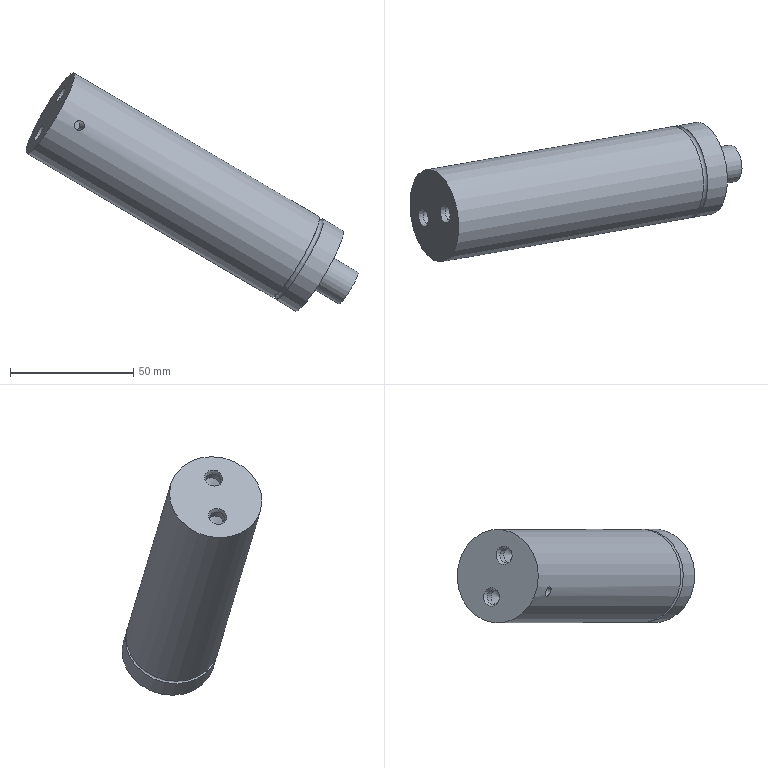Part | NX | features solid 2 | 1 solid | 15 faces | box 134.944 x 56.817 x 96.909 mm | volume 146987 mm3 | cylinder 7 | cone 4 | plane 3 | torus 1 | commonest cylinder face diameters 6 x2 38 x2 4 x1 15 x1 18 x1
STEP:
#1=CARTESIAN_POINT('',(878.455,397.185,19.862));
#2=VERTEX_POINT('',#1);
#3=CARTESIAN_POINT('',(877.303,397.035,18.721));
#4=CARTESIAN_POINT('',(878.645,397.191,19.754));
#5=CARTESIAN_POINT('',(878.849,397.307,21.436));
#6=CARTESIAN_POINT('',(877.82,397.207,22.781));
#7=CARTESIAN_POINT('',(876.177,396.836,23.005));
#8=CARTESIAN_POINT('',(874.865,396.525,21.972));
#9=CARTESIAN_POINT('',(874.632,396.564,20.293));
#10=CARTESIAN_POINT('',(875.633,396.821,18.945));
#11=CARTESIAN_POINT('',(877.303,397.035,18.721));
#12=CARTESIAN_POINT('',(878.645,397.191,19.754));
#13=CARTESIAN_POINT('',(878.849,397.307,21.436));
#14=B_SPLINE_CURVE_WITH_KNOTS('',3,(#3,#4,#5,#6,#7,#8,#9,#10,#11,#12,#13),.UNSPECIFIED.,.T.,.F.,(1,1,1,1,1,1,1,1,1,1,1,1,1,1,1),(-0.004692,-0.003128,-0.001564,0.,0.001564,0.003128,0.004692,0.006257,0.007821,0.009385,0.01095,0.01251,0.01408,0.01564,0.01721),.UNSPECIFIED.);
#15=EDGE_CURVE('',#2,#2,#14,.T.);
#16=ORIENTED_EDGE('',*,*,#15,.F.);
#17=EDGE_LOOP('',(#16));
#18=FACE_BOUND('',#17,.T.);
#19=CARTESIAN_POINT('',(855.566,412.442,9.408));
#20=VERTEX_POINT('',#19);
#21=CARTESIAN_POINT('',(864.922,414.091,25.863));
#22=DIRECTION('',(0.8529,0.1504,-0.5));
#23=DIRECTION('',(-0.4924,-0.08682,-0.866));
#24=AXIS2_PLACEMENT_3D('',#21,#22,#23);
#25=CIRCLE('',#24,19.);
#26=EDGE_CURVE('',#20,#20,#25,.T.);
#27=ORIENTED_EDGE('',*,*,#26,.T.);
#28=EDGE_LOOP('',(#27));
#29=FACE_BOUND('',#28,.T.);
#30=CARTESIAN_POINT('',(955.011,429.976,-48.892));
#31=VERTEX_POINT('',#30);
#32=CARTESIAN_POINT('',(964.366,431.626,-32.437));
#33=DIRECTION('',(0.8529,0.1504,-0.5));
#34=DIRECTION('',(-0.4924,-0.08682,-0.866));
#35=AXIS2_PLACEMENT_3D('',#32,#33,#34);
#36=CIRCLE('',#35,19.);
#37=EDGE_CURVE('',#31,#31,#36,.T.);
#38=ORIENTED_EDGE('',*,*,#37,.F.);
#39=EDGE_LOOP('',(#38));
#40=FACE_BOUND('',#39,.T.);
#41=CARTESIAN_POINT('',(972.81,433.115,-37.387));
#42=DIRECTION('',(-0.8529,-0.1504,0.5));
#43=DIRECTION('',(0.4924,0.08682,0.866));
#44=AXIS2_PLACEMENT_3D('',#41,#42,#43);
#45=CYLINDRICAL_SURFACE('',#44,19.);
#46=ADVANCED_FACE('',(#18,#29,#40),#45,.T.);
#47=CARTESIAN_POINT('',(867.507,414.547,30.41));
#48=VERTEX_POINT('',#47);
#49=CARTESIAN_POINT('',(869.353,414.873,33.657));
#50=DIRECTION('',(-0.8529,-0.1504,0.5));
#51=DIRECTION('',(-0.4924,-0.08682,-0.866));
#52=AXIS2_PLACEMENT_3D('',#49,#50,#51);
#53=CIRCLE('',#52,3.75);
#54=EDGE_CURVE('',#48,#48,#53,.T.);
#55=ORIENTED_EDGE('',*,*,#54,.F.);
#56=EDGE_LOOP('',(#55));
#57=FACE_BOUND('',#56,.T.);
#58=CARTESIAN_POINT('',(858.644,412.984,14.821));
#59=VERTEX_POINT('',#58);
#60=CARTESIAN_POINT('',(860.49,413.31,18.069));
#61=DIRECTION('',(-0.8529,-0.1504,0.5));
#62=DIRECTION('',(-0.4924,-0.08682,-0.866));
#63=AXIS2_PLACEMENT_3D('',#60,#61,#62);
#64=CIRCLE('',#63,3.75);
#65=EDGE_CURVE('',#59,#59,#64,.T.);
#66=ORIENTED_EDGE('',*,*,#65,.F.);
#67=EDGE_LOOP('',(#66));
#68=FACE_BOUND('',#67,.T.);
#69=ORIENTED_EDGE('',*,*,#26,.F.);
#70=EDGE_LOOP('',(#69));
#71=FACE_BOUND('',#70,.T.);
#72=CARTESIAN_POINT('',(864.922,414.091,25.863));
#73=DIRECTION('',(-0.8529,-0.1504,0.5));
#74=DIRECTION('',(0.4924,0.08682,0.866));
#75=AXIS2_PLACEMENT_3D('',#72,#73,#74);
#76=PLANE('',#75);
#77=ADVANCED_FACE('',(#57,#68,#71),#76,.T.);
#78=ORIENTED_EDGE('',*,*,#15,.T.);
#79=EDGE_LOOP('',(#78));
#80=FACE_BOUND('',#79,.T.);
#81=CARTESIAN_POINT('',(876.826,407.055,20.081));
#82=VERTEX_POINT('',#81);
#83=CARTESIAN_POINT('',(877.011,407.239,21.692));
#84=CARTESIAN_POINT('',(877.032,407.036,19.997));
#85=CARTESIAN_POINT('',(875.815,406.945,18.807));
#86=CARTESIAN_POINT('',(874.114,406.854,18.822));
#87=CARTESIAN_POINT('',(872.962,406.524,20.036));
#88=CARTESIAN_POINT('',(873.013,406.328,21.728));
#89=CARTESIAN_POINT('',(874.184,406.657,22.918));
#90=CARTESIAN_POINT('',(875.817,407.155,22.904));
#91=CARTESIAN_POINT('',(877.011,407.239,21.692));
#92=CARTESIAN_POINT('',(877.032,407.036,19.997));
#93=CARTESIAN_POINT('',(875.815,406.945,18.807));
#94=B_SPLINE_CURVE_WITH_KNOTS('',3,(#83,#84,#85,#86,#87,#88,#89,#90,#91,#92,#93),.UNSPECIFIED.,.T.,.F.,(1,1,1,1,1,1,1,1,1,1,1,1,1,1,1),(-0.004704,-0.003136,-0.001568,0.,0.001568,0.003136,0.004704,0.006272,0.00784,0.009408,0.01098,0.01254,0.01411,0.01568,0.01725),.UNSPECIFIED.);
#95=EDGE_CURVE('',#82,#82,#94,.T.);
#96=ORIENTED_EDGE('',*,*,#95,.T.);
#97=EDGE_LOOP('',(#96));
#98=FACE_BOUND('',#97,.T.);
#99=CARTESIAN_POINT('',(879.007,384.081,20.863));
#100=DIRECTION('',(-0.1736,0.9848,0.));
#101=DIRECTION('',(-0.4924,-0.08682,-0.866));
#102=AXIS2_PLACEMENT_3D('',#99,#100,#101);
#103=CYLINDRICAL_SURFACE('',#102,2.);
#104=ADVANCED_FACE('',(#80,#98),#103,.F.);
#105=CARTESIAN_POINT('',(863.277,413.801,12.971));
#106=VERTEX_POINT('',#105);
#107=CARTESIAN_POINT('',(864.755,414.062,15.569));
#108=DIRECTION('',(-0.8529,-0.1504,0.5));
#109=DIRECTION('',(-0.4924,-0.08682,-0.866));
#110=AXIS2_PLACEMENT_3D('',#107,#108,#109);
#111=CIRCLE('',#110,3.);
#112=EDGE_CURVE('',#106,#106,#111,.T.);
#113=ORIENTED_EDGE('',*,*,#112,.T.);
#114=EDGE_LOOP('',(#113));
#115=FACE_BOUND('',#114,.T.);
#116=CARTESIAN_POINT('',(866.292,414.333,14.667));
#117=VERTEX_POINT('',#116);
#118=VERTEX_LOOP('',#117);
#119=FACE_BOUND('',#118,.T.);
#120=CARTESIAN_POINT('',(864.755,414.062,15.569));
#121=DIRECTION('',(-0.8529,-0.1504,0.5));
#122=DIRECTION('',(0.4924,0.08682,0.866));
#123=AXIS2_PLACEMENT_3D('',#120,#121,#122);
#124=CONICAL_SURFACE('',#123,3.,1.03);
#125=ADVANCED_FACE('',(#115,#119),#124,.F.);
#126=ORIENTED_EDGE('',*,*,#112,.F.);
#127=EDGE_LOOP('',(#126));
#128=FACE_BOUND('',#127,.T.);
#129=CARTESIAN_POINT('',(860.557,413.322,14.565));
#130=VERTEX_POINT('',#129);
#131=CARTESIAN_POINT('',(862.034,413.582,17.163));
#132=DIRECTION('',(-0.8529,-0.1504,0.5));
#133=DIRECTION('',(-0.4924,-0.08682,-0.866));
#134=AXIS2_PLACEMENT_3D('',#131,#132,#133);
#135=CIRCLE('',#134,3.);
#136=EDGE_CURVE('',#130,#130,#135,.T.);
#137=ORIENTED_EDGE('',*,*,#136,.T.);
#138=EDGE_LOOP('',(#137));
#139=FACE_BOUND('',#138,.T.);
#140=CARTESIAN_POINT('',(863.475,413.836,16.319));
#141=DIRECTION('',(0.8529,0.1504,-0.5));
#142=DIRECTION('',(-0.4924,-0.08682,-0.866));
#143=AXIS2_PLACEMENT_3D('',#140,#141,#142);
#144=CYLINDRICAL_SURFACE('',#143,3.);
#145=ADVANCED_FACE('',(#128,#139),#144,.F.);
#146=ORIENTED_EDGE('',*,*,#136,.F.);
#147=EDGE_LOOP('',(#146));
#148=FACE_BOUND('',#147,.T.);
#149=ORIENTED_EDGE('',*,*,#65,.T.);
#150=EDGE_LOOP('',(#149));
#151=FACE_BOUND('',#150,.T.);
#152=CARTESIAN_POINT('',(860.49,413.31,18.069));
#153=DIRECTION('',(-0.8529,-0.1504,0.5));
#154=DIRECTION('',(0.4924,0.08682,0.866));
#155=AXIS2_PLACEMENT_3D('',#152,#153,#154);
#156=CONICAL_SURFACE('',#155,3.75,0.3927);
#157=ADVANCED_FACE('',(#148,#151),#156,.F.);
#158=CARTESIAN_POINT('',(872.141,415.364,28.559));
#159=VERTEX_POINT('',#158);
#160=CARTESIAN_POINT('',(873.618,415.625,31.157));
#161=DIRECTION('',(-0.8529,-0.1504,0.5));
#162=DIRECTION('',(-0.4924,-0.08682,-0.866));
#163=AXIS2_PLACEMENT_3D('',#160,#161,#162);
#164=CIRCLE('',#163,3.);
#165=EDGE_CURVE('',#159,#159,#164,.T.);
#166=ORIENTED_EDGE('',*,*,#165,.T.);
#167=EDGE_LOOP('',(#166));
#168=FACE_BOUND('',#167,.T.);
#169=CARTESIAN_POINT('',(875.155,415.896,30.256));
#170=VERTEX_POINT('',#169);
#171=VERTEX_LOOP('',#170);
#172=FACE_BOUND('',#171,.T.);
#173=CARTESIAN_POINT('',(873.618,415.625,31.157));
#174=DIRECTION('',(-0.8529,-0.1504,0.5));
#175=DIRECTION('',(0.4924,0.08682,0.866));
#176=AXIS2_PLACEMENT_3D('',#173,#174,#175);
#177=CONICAL_SURFACE('',#176,3.,1.03);
#178=ADVANCED_FACE('',(#168,#172),#177,.F.);
#179=ORIENTED_EDGE('',*,*,#165,.F.);
#180=EDGE_LOOP('',(#179));
#181=FACE_BOUND('',#180,.T.);
#182=CARTESIAN_POINT('',(869.42,414.885,30.154));
#183=VERTEX_POINT('',#182);
#184=CARTESIAN_POINT('',(870.898,415.145,32.752));
#185=DIRECTION('',(-0.8529,-0.1504,0.5));
#186=DIRECTION('',(-0.4924,-0.08682,-0.866));
#187=AXIS2_PLACEMENT_3D('',#184,#185,#186);
#188=CIRCLE('',#187,3.);
#189=EDGE_CURVE('',#183,#183,#188,.T.);
#190=ORIENTED_EDGE('',*,*,#189,.T.);
#191=EDGE_LOOP('',(#190));
#192=FACE_BOUND('',#191,.T.);
#193=CARTESIAN_POINT('',(872.338,415.399,31.907));
#194=DIRECTION('',(0.8529,0.1504,-0.5));
#195=DIRECTION('',(-0.4924,-0.08682,-0.866));
#196=AXIS2_PLACEMENT_3D('',#193,#194,#195);
#197=CYLINDRICAL_SURFACE('',#196,3.);
#198=ADVANCED_FACE('',(#181,#192),#197,.F.);
#199=ORIENTED_EDGE('',*,*,#189,.F.);
#200=EDGE_LOOP('',(#199));
#201=FACE_BOUND('',#200,.T.);
#202=ORIENTED_EDGE('',*,*,#54,.T.);
#203=EDGE_LOOP('',(#202));
#204=FACE_BOUND('',#203,.T.);
#205=CARTESIAN_POINT('',(869.353,414.873,33.657));
#206=DIRECTION('',(-0.8529,-0.1504,0.5));
#207=DIRECTION('',(0.4924,0.08682,0.866));
#208=AXIS2_PLACEMENT_3D('',#205,#206,#207);
#209=CONICAL_SURFACE('',#208,3.75,0.3927);
#210=ADVANCED_FACE('',(#201,#204),#209,.F.);
#211=CARTESIAN_POINT('',(970.525,432.043,-44.607));
#212=VERTEX_POINT('',#211);
#213=CARTESIAN_POINT('',(974.089,433.34,-38.137));
#214=DIRECTION('',(-0.8529,-0.1504,0.5));
#215=DIRECTION('',(-0.4753,-0.173,-0.8627));
#216=AXIS2_PLACEMENT_3D('',#213,#214,#215);
#217=CIRCLE('',#216,7.5);
#218=EDGE_CURVE('',#212,#212,#217,.F.);
#219=ORIENTED_EDGE('',*,*,#218,.T.);
#220=EDGE_LOOP('',(#219));
#221=FACE_BOUND('',#220,.T.);
#222=CARTESIAN_POINT('',(989.594,436.743,-38.667));
#223=VERTEX_POINT('',#222);
#224=CARTESIAN_POINT('',(986.029,435.446,-45.137));
#225=DIRECTION('',(0.8529,0.1504,-0.5));
#226=DIRECTION('',(0.4753,0.173,0.8627));
#227=AXIS2_PLACEMENT_3D('',#224,#225,#226);
#228=CIRCLE('',#227,7.5);
#229=EDGE_CURVE('',#223,#223,#228,.F.);
#230=ORIENTED_EDGE('',*,*,#229,.T.);
#231=EDGE_LOOP('',(#230));
#232=FACE_BOUND('',#231,.T.);
#233=CARTESIAN_POINT('',(1042.745,445.446,-78.387));
#234=DIRECTION('',(-0.8529,-0.1504,0.5));
#235=DIRECTION('',(0.4924,0.08682,0.866));
#236=AXIS2_PLACEMENT_3D('',#233,#234,#235);
#237=CYLINDRICAL_SURFACE('',#236,7.5);
#238=ADVANCED_FACE('',(#221,#232),#237,.T.);
#239=ORIENTED_EDGE('',*,*,#218,.F.);
#240=EDGE_LOOP('',(#239));
#241=FACE_BOUND('',#240,.T.);
#242=CARTESIAN_POINT('',(964.733,431.691,-54.592));
#243=VERTEX_POINT('',#242);
#244=CARTESIAN_POINT('',(974.089,433.34,-38.137));
#245=DIRECTION('',(0.8529,0.1504,-0.5));
#246=DIRECTION('',(-0.4924,-0.08682,-0.866));
#247=AXIS2_PLACEMENT_3D('',#244,#245,#246);
#248=CIRCLE('',#247,19.);
#249=EDGE_CURVE('',#243,#243,#248,.T.);
#250=ORIENTED_EDGE('',*,*,#249,.T.);
#251=EDGE_LOOP('',(#250));
#252=FACE_BOUND('',#251,.T.);
#253=CARTESIAN_POINT('',(974.089,433.34,-38.137));
#254=DIRECTION('',(-0.8529,-0.1504,0.5));
#255=DIRECTION('',(0.4924,0.08682,0.866));
#256=AXIS2_PLACEMENT_3D('',#253,#254,#255);
#257=PLANE('',#256);
#258=ADVANCED_FACE('',(#241,#252),#257,.F.);
#259=ORIENTED_EDGE('',*,*,#249,.F.);
#260=EDGE_LOOP('',(#259));
#261=FACE_BOUND('',#260,.T.);
#262=CARTESIAN_POINT('',(956.716,430.277,-49.892));
#263=VERTEX_POINT('',#262);
#264=CARTESIAN_POINT('',(966.072,431.927,-33.437));
#265=DIRECTION('',(0.8529,0.1504,-0.5));
#266=DIRECTION('',(-0.4924,-0.08682,-0.866));
#267=AXIS2_PLACEMENT_3D('',#264,#265,#266);
#268=CIRCLE('',#267,19.);
#269=EDGE_CURVE('',#263,#263,#268,.F.);
#270=ORIENTED_EDGE('',*,*,#269,.F.);
#271=EDGE_LOOP('',(#270));
#272=FACE_BOUND('',#271,.T.);
#273=CARTESIAN_POINT('',(972.81,433.115,-37.387));
#274=DIRECTION('',(-0.8529,-0.1504,0.5));
#275=DIRECTION('',(0.4924,0.08682,0.866));
#276=AXIS2_PLACEMENT_3D('',#273,#274,#275);
#277=CYLINDRICAL_SURFACE('',#276,19.);
#278=ADVANCED_FACE('',(#261,#272),#277,.T.);
#279=ORIENTED_EDGE('',*,*,#269,.T.);
#280=EDGE_LOOP('',(#279));
#281=FACE_BOUND('',#280,.T.);
#282=ORIENTED_EDGE('',*,*,#37,.T.);
#283=EDGE_LOOP('',(#282));
#284=FACE_BOUND('',#283,.T.);
#285=CARTESIAN_POINT('',(965.219,431.776,-32.937));
#286=DIRECTION('',(-0.8529,-0.1504,0.5));
#287=DIRECTION('',(-0.4924,-0.08682,-0.866));
#288=AXIS2_PLACEMENT_3D('',#285,#286,#287);
#289=TOROIDAL_SURFACE('',#288,19.,1.);
#290=ADVANCED_FACE('',(#281,#284),#289,.F.);
#291=ORIENTED_EDGE('',*,*,#229,.F.);
#292=EDGE_LOOP('',(#291));
#293=FACE_BOUND('',#292,.T.);
#294=CARTESIAN_POINT('',(1110.194,-225.535,-32.147));
#295=DIRECTION('',(0.8529,0.1504,-0.5));
#296=DIRECTION('',(-0.1736,0.9848,0.));
#297=AXIS2_PLACEMENT_3D('',#294,#295,#296);
#298=PLANE('',#297);
#299=ADVANCED_FACE('',(#293),#298,.T.);
#300=ORIENTED_EDGE('',*,*,#95,.F.);
#301=EDGE_LOOP('',(#300));
#302=FACE_BOUND('',#301,.T.);
#303=CARTESIAN_POINT('',(897.757,419.881,6.613));
#304=DIRECTION('',(-0.8529,-0.1504,0.5));
#305=DIRECTION('',(-0.4924,-0.08682,-0.866));
#306=AXIS2_PLACEMENT_3D('',#303,#304,#305);
#307=CYLINDRICAL_SURFACE('',#306,9.);
#308=ADVANCED_FACE('',(#302),#307,.T.);
#309=CLOSED_SHELL('',(#46,#77,#104,#125,#145,#157,#178,#198,#210,#238,#258,#278,#290,#299,#308));
#310=MANIFOLD_SOLID_BREP('',#309);
#311=(LENGTH_UNIT()NAMED_UNIT(*)SI_UNIT(.MILLI.,.METRE.));
#312=UNCERTAINTY_MEASURE_WITH_UNIT(LENGTH_MEASURE(0.0508),#311,'','');
#313=(NAMED_UNIT(*)PLANE_ANGLE_UNIT()SI_UNIT($,.RADIAN.));
#314=(NAMED_UNIT(*)SI_UNIT($,.STERADIAN.)SOLID_ANGLE_UNIT());
#315=(GEOMETRIC_REPRESENTATION_CONTEXT(3)GLOBAL_UNCERTAINTY_ASSIGNED_CONTEXT((#312))GLOBAL_UNIT_ASSIGNED_CONTEXT((#311,#313,#314))REPRESENTATION_CONTEXT('',''));
#316=ADVANCED_BREP_SHAPE_REPRESENTATION('',(#310),#315);